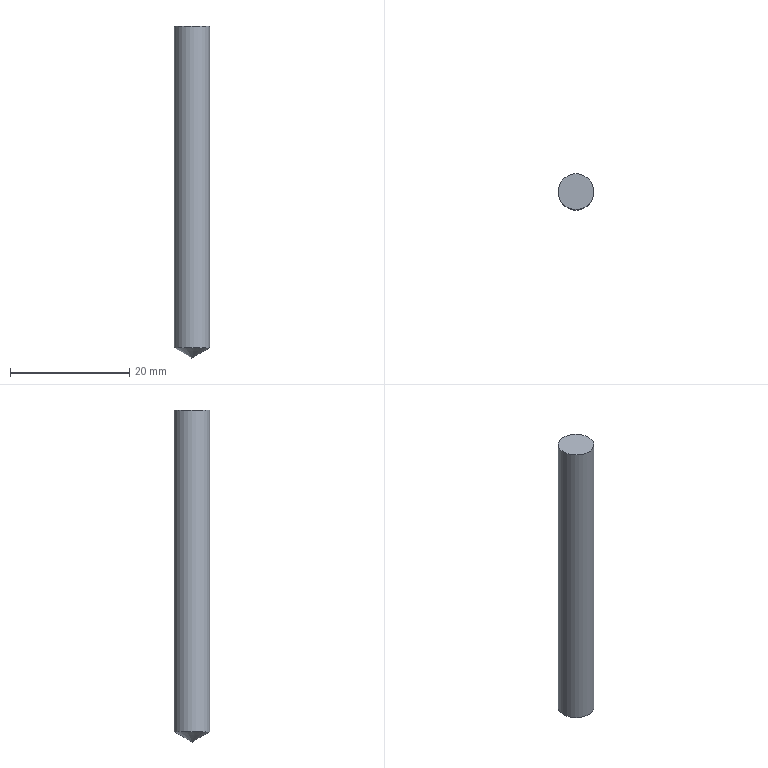Part | NX | features solid 2 | 1 solid | 3 faces | box 6 x 6 x 55.732 mm | volume 1543 mm3 | cylinder 1 | plane 1 | cone 1 | commonest cylinder face diameters 6 x1
STEP:
#1=CARTESIAN_POINT('',(82.,35.,-154.));
#2=VERTEX_POINT('',#1);
#3=CARTESIAN_POINT('',(85.,35.,-154.));
#4=DIRECTION('',(0.,0.,-1.));
#5=DIRECTION('',(-1.,0.,0.));
#6=AXIS2_PLACEMENT_3D('',#3,#4,#5);
#7=CIRCLE('',#6,3.);
#8=EDGE_CURVE('',#2,#2,#7,.T.);
#9=ORIENTED_EDGE('',*,*,#8,.F.);
#10=EDGE_LOOP('',(#9));
#11=FACE_BOUND('',#10,.T.);
#12=CARTESIAN_POINT('',(82.,35.,-100.));
#13=VERTEX_POINT('',#12);
#14=CARTESIAN_POINT('',(85.,35.,-100.));
#15=DIRECTION('',(0.,0.,-1.));
#16=DIRECTION('',(-1.,0.,0.));
#17=AXIS2_PLACEMENT_3D('',#14,#15,#16);
#18=CIRCLE('',#17,3.);
#19=EDGE_CURVE('',#13,#13,#18,.T.);
#20=ORIENTED_EDGE('',*,*,#19,.T.);
#21=EDGE_LOOP('',(#20));
#22=FACE_BOUND('',#21,.T.);
#23=CARTESIAN_POINT('',(85.,35.,-150.));
#24=DIRECTION('',(0.,0.,1.));
#25=DIRECTION('',(1.,0.,0.));
#26=AXIS2_PLACEMENT_3D('',#23,#24,#25);
#27=CYLINDRICAL_SURFACE('',#26,3.);
#28=ADVANCED_FACE('',(#11,#22),#27,.T.);
#29=ORIENTED_EDGE('',*,*,#19,.F.);
#30=EDGE_LOOP('',(#29));
#31=FACE_BOUND('',#30,.T.);
#32=CARTESIAN_POINT('',(85.,35.,-100.));
#33=DIRECTION('',(0.,0.,-1.));
#34=DIRECTION('',(-1.,0.,0.));
#35=AXIS2_PLACEMENT_3D('',#32,#33,#34);
#36=PLANE('',#35);
#37=ADVANCED_FACE('',(#31),#36,.F.);
#38=ORIENTED_EDGE('',*,*,#8,.T.);
#39=EDGE_LOOP('',(#38));
#40=FACE_BOUND('',#39,.T.);
#41=CARTESIAN_POINT('',(85.,35.,-155.732));
#42=VERTEX_POINT('',#41);
#43=VERTEX_LOOP('',#42);
#44=FACE_BOUND('',#43,.T.);
#45=CARTESIAN_POINT('',(85.,35.,-155.732));
#46=DIRECTION('',(0.,0.,1.));
#47=DIRECTION('',(1.,0.,0.));
#48=AXIS2_PLACEMENT_3D('',#45,#46,#47);
#49=CONICAL_SURFACE('',#48,0.,1.047);
#50=ADVANCED_FACE('',(#40,#44),#49,.T.);
#51=CLOSED_SHELL('',(#28,#37,#50));
#52=MANIFOLD_SOLID_BREP('',#51);
#53=(LENGTH_UNIT()NAMED_UNIT(*)SI_UNIT(.MILLI.,.METRE.));
#54=UNCERTAINTY_MEASURE_WITH_UNIT(LENGTH_MEASURE(0.00001),#53,'','');
#55=(NAMED_UNIT(*)PLANE_ANGLE_UNIT()SI_UNIT($,.RADIAN.));
#56=(NAMED_UNIT(*)SI_UNIT($,.STERADIAN.)SOLID_ANGLE_UNIT());
#57=(GEOMETRIC_REPRESENTATION_CONTEXT(3)GLOBAL_UNCERTAINTY_ASSIGNED_CONTEXT((#54))GLOBAL_UNIT_ASSIGNED_CONTEXT((#53,#55,#56))REPRESENTATION_CONTEXT('',''));
#58=ADVANCED_BREP_SHAPE_REPRESENTATION('',(#52),#57);